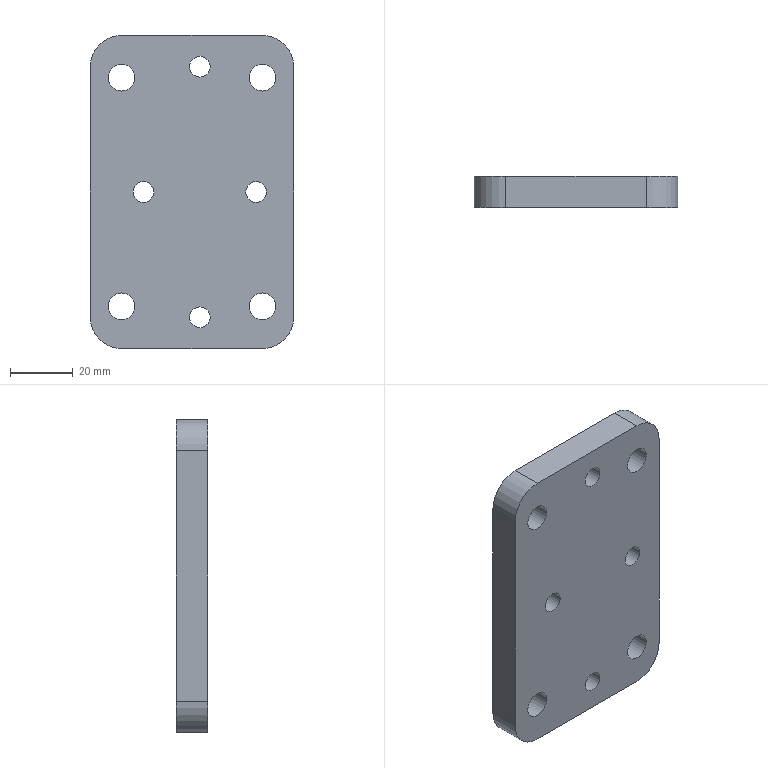Part | STEP file | JBJ-P-1006-11 | 1 solid | 22 faces | box 65 x 10 x 100 mm | volume 59980 mm3 | cylinder 12 | plane 6 | cone 4 | commonest cylinder face diameters 6.6 x4 8.5 x4 20 x4
STEP:
#1=CARTESIAN_POINT('',(0.,0.,10.));
#2=VERTEX_POINT('',#1);
#3=CARTESIAN_POINT('',(0.,0.,90.));
#4=VERTEX_POINT('',#3);
#5=CARTESIAN_POINT('',(0.,0.,0.));
#6=DIRECTION('',(0.,0.,1.));
#7=VECTOR('',#6,1000.);
#8=LINE('',#5,#7);
#9=EDGE_CURVE('',#2,#4,#8,.T.);
#10=ORIENTED_EDGE('',*,*,#9,.T.);
#11=CARTESIAN_POINT('',(0.,10.,90.));
#12=VERTEX_POINT('',#11);
#13=CARTESIAN_POINT('',(0.,10.,90.));
#14=DIRECTION('',(0.,1.,0.));
#15=VECTOR('',#14,1000.);
#16=LINE('',#13,#15);
#17=EDGE_CURVE('',#4,#12,#16,.T.);
#18=ORIENTED_EDGE('',*,*,#17,.T.);
#19=CARTESIAN_POINT('',(0.,10.,10.));
#20=VERTEX_POINT('',#19);
#21=CARTESIAN_POINT('',(0.,10.,0.));
#22=DIRECTION('',(0.,0.,1.));
#23=VECTOR('',#22,1000.);
#24=LINE('',#21,#23);
#25=EDGE_CURVE('',#20,#12,#24,.T.);
#26=ORIENTED_EDGE('',*,*,#25,.F.);
#27=CARTESIAN_POINT('',(0.,10.,10.));
#28=DIRECTION('',(0.,-1.,0.));
#29=VECTOR('',#28,1000.);
#30=LINE('',#27,#29);
#31=EDGE_CURVE('',#20,#2,#30,.T.);
#32=ORIENTED_EDGE('',*,*,#31,.T.);
#33=EDGE_LOOP('',(#10,#18,#26,#32));
#34=FACE_OUTER_BOUND('',#33,.T.);
#35=CARTESIAN_POINT('',(0.,10.,0.));
#36=DIRECTION('',(1.,0.,0.));
#37=DIRECTION('',(0.,0.,-1.));
#38=AXIS2_PLACEMENT_3D('',#35,#36,#37);
#39=PLANE('',#38);
#40=ADVANCED_FACE('',(#34),#39,.F.);
#41=CARTESIAN_POINT('',(10.,10.,100.));
#42=VERTEX_POINT('',#41);
#43=CARTESIAN_POINT('',(55.,10.,100.));
#44=VERTEX_POINT('',#43);
#45=CARTESIAN_POINT('',(0.,10.,100.));
#46=DIRECTION('',(1.,0.,0.));
#47=VECTOR('',#46,1000.);
#48=LINE('',#45,#47);
#49=EDGE_CURVE('',#42,#44,#48,.T.);
#50=ORIENTED_EDGE('',*,*,#49,.F.);
#51=CARTESIAN_POINT('',(10.,0.,100.));
#52=VERTEX_POINT('',#51);
#53=CARTESIAN_POINT('',(10.,10.,100.));
#54=DIRECTION('',(0.,-1.,0.));
#55=VECTOR('',#54,1000.);
#56=LINE('',#53,#55);
#57=EDGE_CURVE('',#42,#52,#56,.T.);
#58=ORIENTED_EDGE('',*,*,#57,.T.);
#59=CARTESIAN_POINT('',(55.,0.,100.));
#60=VERTEX_POINT('',#59);
#61=CARTESIAN_POINT('',(0.,0.,100.));
#62=DIRECTION('',(1.,0.,0.));
#63=VECTOR('',#62,1000.);
#64=LINE('',#61,#63);
#65=EDGE_CURVE('',#52,#60,#64,.T.);
#66=ORIENTED_EDGE('',*,*,#65,.T.);
#67=CARTESIAN_POINT('',(55.,10.,100.));
#68=DIRECTION('',(0.,1.,0.));
#69=VECTOR('',#68,1000.);
#70=LINE('',#67,#69);
#71=EDGE_CURVE('',#60,#44,#70,.T.);
#72=ORIENTED_EDGE('',*,*,#71,.T.);
#73=EDGE_LOOP('',(#50,#58,#66,#72));
#74=FACE_OUTER_BOUND('',#73,.T.);
#75=CARTESIAN_POINT('',(0.,10.,100.));
#76=DIRECTION('',(0.,0.,-1.));
#77=DIRECTION('',(-1.,0.,0.));
#78=AXIS2_PLACEMENT_3D('',#75,#76,#77);
#79=PLANE('',#78);
#80=ADVANCED_FACE('',(#74),#79,.F.);
#81=CARTESIAN_POINT('',(65.,10.,90.));
#82=VERTEX_POINT('',#81);
#83=CARTESIAN_POINT('',(65.,10.,10.));
#84=VERTEX_POINT('',#83);
#85=CARTESIAN_POINT('',(65.,10.,0.));
#86=DIRECTION('',(0.,0.,-1.));
#87=VECTOR('',#86,1000.);
#88=LINE('',#85,#87);
#89=EDGE_CURVE('',#82,#84,#88,.T.);
#90=ORIENTED_EDGE('',*,*,#89,.F.);
#91=CARTESIAN_POINT('',(65.,0.,90.));
#92=VERTEX_POINT('',#91);
#93=CARTESIAN_POINT('',(65.,10.,90.));
#94=DIRECTION('',(0.,-1.,0.));
#95=VECTOR('',#94,1000.);
#96=LINE('',#93,#95);
#97=EDGE_CURVE('',#82,#92,#96,.T.);
#98=ORIENTED_EDGE('',*,*,#97,.T.);
#99=CARTESIAN_POINT('',(65.,0.,10.));
#100=VERTEX_POINT('',#99);
#101=CARTESIAN_POINT('',(65.,0.,0.));
#102=DIRECTION('',(0.,0.,-1.));
#103=VECTOR('',#102,1000.);
#104=LINE('',#101,#103);
#105=EDGE_CURVE('',#92,#100,#104,.T.);
#106=ORIENTED_EDGE('',*,*,#105,.T.);
#107=CARTESIAN_POINT('',(65.,10.,10.));
#108=DIRECTION('',(0.,1.,0.));
#109=VECTOR('',#108,1000.);
#110=LINE('',#107,#109);
#111=EDGE_CURVE('',#100,#84,#110,.T.);
#112=ORIENTED_EDGE('',*,*,#111,.T.);
#113=EDGE_LOOP('',(#90,#98,#106,#112));
#114=FACE_OUTER_BOUND('',#113,.T.);
#115=CARTESIAN_POINT('',(65.,10.,0.));
#116=DIRECTION('',(-1.,0.,0.));
#117=DIRECTION('',(0.,0.,1.));
#118=AXIS2_PLACEMENT_3D('',#115,#116,#117);
#119=PLANE('',#118);
#120=ADVANCED_FACE('',(#114),#119,.F.);
#121=CARTESIAN_POINT('',(55.,10.,0.));
#122=VERTEX_POINT('',#121);
#123=CARTESIAN_POINT('',(10.,10.,0.));
#124=VERTEX_POINT('',#123);
#125=CARTESIAN_POINT('',(0.,10.,0.));
#126=DIRECTION('',(-1.,0.,0.));
#127=VECTOR('',#126,1000.);
#128=LINE('',#125,#127);
#129=EDGE_CURVE('',#122,#124,#128,.T.);
#130=ORIENTED_EDGE('',*,*,#129,.F.);
#131=CARTESIAN_POINT('',(55.,0.,0.));
#132=VERTEX_POINT('',#131);
#133=CARTESIAN_POINT('',(55.,10.,0.));
#134=DIRECTION('',(0.,-1.,0.));
#135=VECTOR('',#134,1000.);
#136=LINE('',#133,#135);
#137=EDGE_CURVE('',#122,#132,#136,.T.);
#138=ORIENTED_EDGE('',*,*,#137,.T.);
#139=CARTESIAN_POINT('',(10.,0.,0.));
#140=VERTEX_POINT('',#139);
#141=CARTESIAN_POINT('',(0.,0.,0.));
#142=DIRECTION('',(-1.,0.,0.));
#143=VECTOR('',#142,1000.);
#144=LINE('',#141,#143);
#145=EDGE_CURVE('',#132,#140,#144,.T.);
#146=ORIENTED_EDGE('',*,*,#145,.T.);
#147=CARTESIAN_POINT('',(10.,10.,0.));
#148=DIRECTION('',(0.,1.,0.));
#149=VECTOR('',#148,1000.);
#150=LINE('',#147,#149);
#151=EDGE_CURVE('',#140,#124,#150,.T.);
#152=ORIENTED_EDGE('',*,*,#151,.T.);
#153=EDGE_LOOP('',(#130,#138,#146,#152));
#154=FACE_OUTER_BOUND('',#153,.T.);
#155=CARTESIAN_POINT('',(0.,10.,0.));
#156=DIRECTION('',(0.,0.,1.));
#157=DIRECTION('',(1.,0.,0.));
#158=AXIS2_PLACEMENT_3D('',#155,#156,#157);
#159=PLANE('',#158);
#160=ADVANCED_FACE('',(#154),#159,.F.);
#161=CARTESIAN_POINT('',(17.,10.,56.4));
#162=VERTEX_POINT('',#161);
#163=CARTESIAN_POINT('',(17.,10.,50.));
#164=DIRECTION('',(0.,1.,0.));
#165=DIRECTION('',(0.,0.,1.));
#166=AXIS2_PLACEMENT_3D('',#163,#164,#165);
#167=CIRCLE('',#166,6.4);
#168=EDGE_CURVE('',#162,#162,#167,.T.);
#169=ORIENTED_EDGE('',*,*,#168,.F.);
#170=EDGE_LOOP('',(#169));
#171=FACE_BOUND('',#170,.T.);
#172=CARTESIAN_POINT('',(35.,10.,16.4));
#173=VERTEX_POINT('',#172);
#174=CARTESIAN_POINT('',(35.,10.,10.));
#175=DIRECTION('',(0.,1.,0.));
#176=DIRECTION('',(0.,0.,1.));
#177=AXIS2_PLACEMENT_3D('',#174,#175,#176);
#178=CIRCLE('',#177,6.4);
#179=EDGE_CURVE('',#173,#173,#178,.T.);
#180=ORIENTED_EDGE('',*,*,#179,.F.);
#181=EDGE_LOOP('',(#180));
#182=FACE_BOUND('',#181,.T.);
#183=CARTESIAN_POINT('',(35.,10.,96.4));
#184=VERTEX_POINT('',#183);
#185=CARTESIAN_POINT('',(35.,10.,90.));
#186=DIRECTION('',(0.,1.,0.));
#187=DIRECTION('',(0.,0.,1.));
#188=AXIS2_PLACEMENT_3D('',#185,#186,#187);
#189=CIRCLE('',#188,6.4);
#190=EDGE_CURVE('',#184,#184,#189,.T.);
#191=ORIENTED_EDGE('',*,*,#190,.F.);
#192=EDGE_LOOP('',(#191));
#193=FACE_BOUND('',#192,.T.);
#194=CARTESIAN_POINT('',(53.,10.,56.4));
#195=VERTEX_POINT('',#194);
#196=CARTESIAN_POINT('',(53.,10.,50.));
#197=DIRECTION('',(0.,1.,0.));
#198=DIRECTION('',(0.,0.,1.));
#199=AXIS2_PLACEMENT_3D('',#196,#197,#198);
#200=CIRCLE('',#199,6.4);
#201=EDGE_CURVE('',#195,#195,#200,.T.);
#202=ORIENTED_EDGE('',*,*,#201,.F.);
#203=EDGE_LOOP('',(#202));
#204=FACE_BOUND('',#203,.T.);
#205=CARTESIAN_POINT('',(10.,10.,17.75));
#206=VERTEX_POINT('',#205);
#207=CARTESIAN_POINT('',(10.,10.,13.5));
#208=DIRECTION('',(0.,1.,0.));
#209=DIRECTION('',(0.,0.,1.));
#210=AXIS2_PLACEMENT_3D('',#207,#208,#209);
#211=CIRCLE('',#210,4.25);
#212=EDGE_CURVE('',#206,#206,#211,.T.);
#213=ORIENTED_EDGE('',*,*,#212,.F.);
#214=EDGE_LOOP('',(#213));
#215=FACE_BOUND('',#214,.T.);
#216=CARTESIAN_POINT('',(55.,10.,17.75));
#217=VERTEX_POINT('',#216);
#218=CARTESIAN_POINT('',(55.,10.,13.5));
#219=DIRECTION('',(0.,1.,0.));
#220=DIRECTION('',(0.,0.,1.));
#221=AXIS2_PLACEMENT_3D('',#218,#219,#220);
#222=CIRCLE('',#221,4.25);
#223=EDGE_CURVE('',#217,#217,#222,.T.);
#224=ORIENTED_EDGE('',*,*,#223,.F.);
#225=EDGE_LOOP('',(#224));
#226=FACE_BOUND('',#225,.T.);
#227=CARTESIAN_POINT('',(55.,10.,90.75));
#228=VERTEX_POINT('',#227);
#229=CARTESIAN_POINT('',(55.,10.,86.5));
#230=DIRECTION('',(0.,1.,0.));
#231=DIRECTION('',(0.,0.,1.));
#232=AXIS2_PLACEMENT_3D('',#229,#230,#231);
#233=CIRCLE('',#232,4.25);
#234=EDGE_CURVE('',#228,#228,#233,.T.);
#235=ORIENTED_EDGE('',*,*,#234,.F.);
#236=EDGE_LOOP('',(#235));
#237=FACE_BOUND('',#236,.T.);
#238=CARTESIAN_POINT('',(10.,10.,90.75));
#239=VERTEX_POINT('',#238);
#240=CARTESIAN_POINT('',(10.,10.,86.5));
#241=DIRECTION('',(0.,1.,0.));
#242=DIRECTION('',(0.,0.,1.));
#243=AXIS2_PLACEMENT_3D('',#240,#241,#242);
#244=CIRCLE('',#243,4.25);
#245=EDGE_CURVE('',#239,#239,#244,.T.);
#246=ORIENTED_EDGE('',*,*,#245,.F.);
#247=EDGE_LOOP('',(#246));
#248=FACE_BOUND('',#247,.T.);
#249=ORIENTED_EDGE('',*,*,#25,.T.);
#250=CARTESIAN_POINT('',(10.,10.,90.));
#251=DIRECTION('',(0.,1.,0.));
#252=DIRECTION('',(0.,0.,1.));
#253=AXIS2_PLACEMENT_3D('',#250,#251,#252);
#254=CIRCLE('',#253,10.);
#255=EDGE_CURVE('',#12,#42,#254,.T.);
#256=ORIENTED_EDGE('',*,*,#255,.T.);
#257=ORIENTED_EDGE('',*,*,#49,.T.);
#258=CARTESIAN_POINT('',(55.,10.,90.));
#259=DIRECTION('',(0.,1.,0.));
#260=DIRECTION('',(0.,0.,1.));
#261=AXIS2_PLACEMENT_3D('',#258,#259,#260);
#262=CIRCLE('',#261,10.);
#263=EDGE_CURVE('',#44,#82,#262,.T.);
#264=ORIENTED_EDGE('',*,*,#263,.T.);
#265=ORIENTED_EDGE('',*,*,#89,.T.);
#266=CARTESIAN_POINT('',(55.,10.,10.));
#267=DIRECTION('',(0.,1.,0.));
#268=DIRECTION('',(0.,0.,1.));
#269=AXIS2_PLACEMENT_3D('',#266,#267,#268);
#270=CIRCLE('',#269,10.);
#271=EDGE_CURVE('',#84,#122,#270,.T.);
#272=ORIENTED_EDGE('',*,*,#271,.T.);
#273=ORIENTED_EDGE('',*,*,#129,.T.);
#274=CARTESIAN_POINT('',(10.,10.,10.));
#275=DIRECTION('',(0.,1.,0.));
#276=DIRECTION('',(0.,0.,1.));
#277=AXIS2_PLACEMENT_3D('',#274,#275,#276);
#278=CIRCLE('',#277,10.);
#279=EDGE_CURVE('',#124,#20,#278,.T.);
#280=ORIENTED_EDGE('',*,*,#279,.T.);
#281=EDGE_LOOP('',(#249,#256,#257,#264,#265,#272,#273,#280));
#282=FACE_OUTER_BOUND('',#281,.T.);
#283=CARTESIAN_POINT('',(0.,10.,0.));
#284=DIRECTION('',(0.,1.,0.));
#285=DIRECTION('',(0.,0.,1.));
#286=AXIS2_PLACEMENT_3D('',#283,#284,#285);
#287=PLANE('',#286);
#288=ADVANCED_FACE('',(#171,#182,#193,#204,#215,#226,#237,#248,#282),#287,.T.);
#289=CARTESIAN_POINT('',(17.,0.,53.3));
#290=VERTEX_POINT('',#289);
#291=CARTESIAN_POINT('',(17.,0.,50.));
#292=DIRECTION('',(0.,1.,0.));
#293=DIRECTION('',(0.,0.,1.));
#294=AXIS2_PLACEMENT_3D('',#291,#292,#293);
#295=CIRCLE('',#294,3.3);
#296=EDGE_CURVE('',#290,#290,#295,.T.);
#297=ORIENTED_EDGE('',*,*,#296,.T.);
#298=EDGE_LOOP('',(#297));
#299=FACE_BOUND('',#298,.T.);
#300=CARTESIAN_POINT('',(35.,0.,13.3));
#301=VERTEX_POINT('',#300);
#302=CARTESIAN_POINT('',(35.,0.,10.));
#303=DIRECTION('',(0.,1.,0.));
#304=DIRECTION('',(0.,0.,1.));
#305=AXIS2_PLACEMENT_3D('',#302,#303,#304);
#306=CIRCLE('',#305,3.3);
#307=EDGE_CURVE('',#301,#301,#306,.T.);
#308=ORIENTED_EDGE('',*,*,#307,.T.);
#309=EDGE_LOOP('',(#308));
#310=FACE_BOUND('',#309,.T.);
#311=CARTESIAN_POINT('',(35.,0.,93.3));
#312=VERTEX_POINT('',#311);
#313=CARTESIAN_POINT('',(35.,0.,90.));
#314=DIRECTION('',(0.,1.,0.));
#315=DIRECTION('',(0.,0.,1.));
#316=AXIS2_PLACEMENT_3D('',#313,#314,#315);
#317=CIRCLE('',#316,3.3);
#318=EDGE_CURVE('',#312,#312,#317,.T.);
#319=ORIENTED_EDGE('',*,*,#318,.T.);
#320=EDGE_LOOP('',(#319));
#321=FACE_BOUND('',#320,.T.);
#322=CARTESIAN_POINT('',(53.,0.,53.3));
#323=VERTEX_POINT('',#322);
#324=CARTESIAN_POINT('',(53.,0.,50.));
#325=DIRECTION('',(0.,1.,0.));
#326=DIRECTION('',(0.,0.,1.));
#327=AXIS2_PLACEMENT_3D('',#324,#325,#326);
#328=CIRCLE('',#327,3.3);
#329=EDGE_CURVE('',#323,#323,#328,.T.);
#330=ORIENTED_EDGE('',*,*,#329,.T.);
#331=EDGE_LOOP('',(#330));
#332=FACE_BOUND('',#331,.T.);
#333=CARTESIAN_POINT('',(10.,0.,17.75));
#334=VERTEX_POINT('',#333);
#335=CARTESIAN_POINT('',(10.,0.,13.5));
#336=DIRECTION('',(0.,1.,0.));
#337=DIRECTION('',(0.,0.,1.));
#338=AXIS2_PLACEMENT_3D('',#335,#336,#337);
#339=CIRCLE('',#338,4.25);
#340=EDGE_CURVE('',#334,#334,#339,.T.);
#341=ORIENTED_EDGE('',*,*,#340,.T.);
#342=EDGE_LOOP('',(#341));
#343=FACE_BOUND('',#342,.T.);
#344=CARTESIAN_POINT('',(55.,0.,17.75));
#345=VERTEX_POINT('',#344);
#346=CARTESIAN_POINT('',(55.,0.,13.5));
#347=DIRECTION('',(0.,1.,0.));
#348=DIRECTION('',(0.,0.,1.));
#349=AXIS2_PLACEMENT_3D('',#346,#347,#348);
#350=CIRCLE('',#349,4.25);
#351=EDGE_CURVE('',#345,#345,#350,.T.);
#352=ORIENTED_EDGE('',*,*,#351,.T.);
#353=EDGE_LOOP('',(#352));
#354=FACE_BOUND('',#353,.T.);
#355=CARTESIAN_POINT('',(55.,0.,90.75));
#356=VERTEX_POINT('',#355);
#357=CARTESIAN_POINT('',(55.,0.,86.5));
#358=DIRECTION('',(0.,1.,0.));
#359=DIRECTION('',(0.,0.,1.));
#360=AXIS2_PLACEMENT_3D('',#357,#358,#359);
#361=CIRCLE('',#360,4.25);
#362=EDGE_CURVE('',#356,#356,#361,.T.);
#363=ORIENTED_EDGE('',*,*,#362,.T.);
#364=EDGE_LOOP('',(#363));
#365=FACE_BOUND('',#364,.T.);
#366=CARTESIAN_POINT('',(10.,0.,90.75));
#367=VERTEX_POINT('',#366);
#368=CARTESIAN_POINT('',(10.,0.,86.5));
#369=DIRECTION('',(0.,1.,0.));
#370=DIRECTION('',(0.,0.,1.));
#371=AXIS2_PLACEMENT_3D('',#368,#369,#370);
#372=CIRCLE('',#371,4.25);
#373=EDGE_CURVE('',#367,#367,#372,.T.);
#374=ORIENTED_EDGE('',*,*,#373,.T.);
#375=EDGE_LOOP('',(#374));
#376=FACE_BOUND('',#375,.T.);
#377=ORIENTED_EDGE('',*,*,#65,.F.);
#378=CARTESIAN_POINT('',(10.,0.,90.));
#379=DIRECTION('',(0.,-1.,0.));
#380=DIRECTION('',(0.,0.,1.));
#381=AXIS2_PLACEMENT_3D('',#378,#379,#380);
#382=CIRCLE('',#381,10.);
#383=EDGE_CURVE('',#52,#4,#382,.T.);
#384=ORIENTED_EDGE('',*,*,#383,.T.);
#385=ORIENTED_EDGE('',*,*,#9,.F.);
#386=CARTESIAN_POINT('',(10.,0.,10.));
#387=DIRECTION('',(0.,-1.,0.));
#388=DIRECTION('',(0.,0.,1.));
#389=AXIS2_PLACEMENT_3D('',#386,#387,#388);
#390=CIRCLE('',#389,10.);
#391=EDGE_CURVE('',#2,#140,#390,.T.);
#392=ORIENTED_EDGE('',*,*,#391,.T.);
#393=ORIENTED_EDGE('',*,*,#145,.F.);
#394=CARTESIAN_POINT('',(55.,0.,10.));
#395=DIRECTION('',(0.,-1.,0.));
#396=DIRECTION('',(0.,0.,1.));
#397=AXIS2_PLACEMENT_3D('',#394,#395,#396);
#398=CIRCLE('',#397,10.);
#399=EDGE_CURVE('',#132,#100,#398,.T.);
#400=ORIENTED_EDGE('',*,*,#399,.T.);
#401=ORIENTED_EDGE('',*,*,#105,.F.);
#402=CARTESIAN_POINT('',(55.,0.,90.));
#403=DIRECTION('',(0.,-1.,0.));
#404=DIRECTION('',(0.,0.,1.));
#405=AXIS2_PLACEMENT_3D('',#402,#403,#404);
#406=CIRCLE('',#405,10.);
#407=EDGE_CURVE('',#92,#60,#406,.T.);
#408=ORIENTED_EDGE('',*,*,#407,.T.);
#409=EDGE_LOOP('',(#377,#384,#385,#392,#393,#400,#401,#408));
#410=FACE_OUTER_BOUND('',#409,.T.);
#411=CARTESIAN_POINT('',(0.,0.,0.));
#412=DIRECTION('',(0.,1.,0.));
#413=DIRECTION('',(0.,0.,1.));
#414=AXIS2_PLACEMENT_3D('',#411,#412,#413);
#415=PLANE('',#414);
#416=ADVANCED_FACE('',(#299,#310,#321,#332,#343,#354,#365,#376,#410),#415,.F.);
#417=ORIENTED_EDGE('',*,*,#255,.F.);
#418=ORIENTED_EDGE('',*,*,#17,.F.);
#419=ORIENTED_EDGE('',*,*,#383,.F.);
#420=ORIENTED_EDGE('',*,*,#57,.F.);
#421=EDGE_LOOP('',(#417,#418,#419,#420));
#422=FACE_OUTER_BOUND('',#421,.T.);
#423=CARTESIAN_POINT('',(10.,10.,90.));
#424=DIRECTION('',(0.,-1.,0.));
#425=DIRECTION('',(0.,0.,-1.));
#426=AXIS2_PLACEMENT_3D('',#423,#424,#425);
#427=CYLINDRICAL_SURFACE('',#426,10.);
#428=ADVANCED_FACE('',(#422),#427,.T.);
#429=ORIENTED_EDGE('',*,*,#263,.F.);
#430=ORIENTED_EDGE('',*,*,#71,.F.);
#431=ORIENTED_EDGE('',*,*,#407,.F.);
#432=ORIENTED_EDGE('',*,*,#97,.F.);
#433=EDGE_LOOP('',(#429,#430,#431,#432));
#434=FACE_OUTER_BOUND('',#433,.T.);
#435=CARTESIAN_POINT('',(55.,10.,90.));
#436=DIRECTION('',(0.,-1.,0.));
#437=DIRECTION('',(0.,0.,-1.));
#438=AXIS2_PLACEMENT_3D('',#435,#436,#437);
#439=CYLINDRICAL_SURFACE('',#438,10.);
#440=ADVANCED_FACE('',(#434),#439,.T.);
#441=ORIENTED_EDGE('',*,*,#271,.F.);
#442=ORIENTED_EDGE('',*,*,#111,.F.);
#443=ORIENTED_EDGE('',*,*,#399,.F.);
#444=ORIENTED_EDGE('',*,*,#137,.F.);
#445=EDGE_LOOP('',(#441,#442,#443,#444));
#446=FACE_OUTER_BOUND('',#445,.T.);
#447=CARTESIAN_POINT('',(55.,10.,10.));
#448=DIRECTION('',(0.,-1.,0.));
#449=DIRECTION('',(0.,0.,-1.));
#450=AXIS2_PLACEMENT_3D('',#447,#448,#449);
#451=CYLINDRICAL_SURFACE('',#450,10.);
#452=ADVANCED_FACE('',(#446),#451,.T.);
#453=ORIENTED_EDGE('',*,*,#279,.F.);
#454=ORIENTED_EDGE('',*,*,#151,.F.);
#455=ORIENTED_EDGE('',*,*,#391,.F.);
#456=ORIENTED_EDGE('',*,*,#31,.F.);
#457=EDGE_LOOP('',(#453,#454,#455,#456));
#458=FACE_OUTER_BOUND('',#457,.T.);
#459=CARTESIAN_POINT('',(10.,10.,10.));
#460=DIRECTION('',(0.,-1.,0.));
#461=DIRECTION('',(0.,0.,-1.));
#462=AXIS2_PLACEMENT_3D('',#459,#460,#461);
#463=CYLINDRICAL_SURFACE('',#462,10.);
#464=ADVANCED_FACE('',(#458),#463,.T.);
#465=ORIENTED_EDGE('',*,*,#245,.T.);
#466=EDGE_LOOP('',(#465));
#467=FACE_OUTER_BOUND('',#466,.T.);
#468=ORIENTED_EDGE('',*,*,#373,.F.);
#469=EDGE_LOOP('',(#468));
#470=FACE_OUTER_BOUND('',#469,.T.);
#471=CARTESIAN_POINT('',(10.,10.,86.5));
#472=DIRECTION('',(0.,1.,0.));
#473=DIRECTION('',(0.,0.,1.));
#474=AXIS2_PLACEMENT_3D('',#471,#472,#473);
#475=CYLINDRICAL_SURFACE('',#474,4.25);
#476=ADVANCED_FACE('',(#467,#470),#475,.F.);
#477=ORIENTED_EDGE('',*,*,#234,.T.);
#478=EDGE_LOOP('',(#477));
#479=FACE_OUTER_BOUND('',#478,.T.);
#480=ORIENTED_EDGE('',*,*,#362,.F.);
#481=EDGE_LOOP('',(#480));
#482=FACE_OUTER_BOUND('',#481,.T.);
#483=CARTESIAN_POINT('',(55.,10.,86.5));
#484=DIRECTION('',(0.,1.,0.));
#485=DIRECTION('',(0.,0.,1.));
#486=AXIS2_PLACEMENT_3D('',#483,#484,#485);
#487=CYLINDRICAL_SURFACE('',#486,4.25);
#488=ADVANCED_FACE('',(#479,#482),#487,.F.);
#489=ORIENTED_EDGE('',*,*,#223,.T.);
#490=EDGE_LOOP('',(#489));
#491=FACE_OUTER_BOUND('',#490,.T.);
#492=ORIENTED_EDGE('',*,*,#351,.F.);
#493=EDGE_LOOP('',(#492));
#494=FACE_OUTER_BOUND('',#493,.T.);
#495=CARTESIAN_POINT('',(55.,10.,13.5));
#496=DIRECTION('',(0.,1.,0.));
#497=DIRECTION('',(0.,0.,1.));
#498=AXIS2_PLACEMENT_3D('',#495,#496,#497);
#499=CYLINDRICAL_SURFACE('',#498,4.25);
#500=ADVANCED_FACE('',(#491,#494),#499,.F.);
#501=ORIENTED_EDGE('',*,*,#212,.T.);
#502=EDGE_LOOP('',(#501));
#503=FACE_OUTER_BOUND('',#502,.T.);
#504=ORIENTED_EDGE('',*,*,#340,.F.);
#505=EDGE_LOOP('',(#504));
#506=FACE_OUTER_BOUND('',#505,.T.);
#507=CARTESIAN_POINT('',(10.,10.,13.5));
#508=DIRECTION('',(0.,1.,0.));
#509=DIRECTION('',(0.,0.,1.));
#510=AXIS2_PLACEMENT_3D('',#507,#508,#509);
#511=CYLINDRICAL_SURFACE('',#510,4.25);
#512=ADVANCED_FACE('',(#503,#506),#511,.F.);
#513=CARTESIAN_POINT('',(53.,6.9,53.3));
#514=VERTEX_POINT('',#513);
#515=CARTESIAN_POINT('',(53.,6.9,50.));
#516=DIRECTION('',(0.,1.,0.));
#517=DIRECTION('',(0.,0.,1.));
#518=AXIS2_PLACEMENT_3D('',#515,#516,#517);
#519=CIRCLE('',#518,3.3);
#520=EDGE_CURVE('',#514,#514,#519,.T.);
#521=ORIENTED_EDGE('',*,*,#520,.T.);
#522=EDGE_LOOP('',(#521));
#523=FACE_OUTER_BOUND('',#522,.T.);
#524=ORIENTED_EDGE('',*,*,#329,.F.);
#525=EDGE_LOOP('',(#524));
#526=FACE_OUTER_BOUND('',#525,.T.);
#527=CARTESIAN_POINT('',(53.,10.,50.));
#528=DIRECTION('',(0.,1.,0.));
#529=DIRECTION('',(0.,0.,1.));
#530=AXIS2_PLACEMENT_3D('',#527,#528,#529);
#531=CYLINDRICAL_SURFACE('',#530,3.3);
#532=ADVANCED_FACE('',(#523,#526),#531,.F.);
#533=ORIENTED_EDGE('',*,*,#520,.F.);
#534=EDGE_LOOP('',(#533));
#535=FACE_BOUND('',#534,.T.);
#536=ORIENTED_EDGE('',*,*,#201,.T.);
#537=EDGE_LOOP('',(#536));
#538=FACE_OUTER_BOUND('',#537,.T.);
#539=CARTESIAN_POINT('',(53.,10.,50.));
#540=DIRECTION('',(0.,1.,0.));
#541=DIRECTION('',(0.,0.,1.));
#542=AXIS2_PLACEMENT_3D('',#539,#540,#541);
#543=CONICAL_SURFACE('',#542,6.4,0.7854);
#544=ADVANCED_FACE('',(#535,#538),#543,.F.);
#545=CARTESIAN_POINT('',(35.,6.9,93.3));
#546=VERTEX_POINT('',#545);
#547=CARTESIAN_POINT('',(35.,6.9,90.));
#548=DIRECTION('',(0.,1.,0.));
#549=DIRECTION('',(0.,0.,1.));
#550=AXIS2_PLACEMENT_3D('',#547,#548,#549);
#551=CIRCLE('',#550,3.3);
#552=EDGE_CURVE('',#546,#546,#551,.T.);
#553=ORIENTED_EDGE('',*,*,#552,.T.);
#554=EDGE_LOOP('',(#553));
#555=FACE_OUTER_BOUND('',#554,.T.);
#556=ORIENTED_EDGE('',*,*,#318,.F.);
#557=EDGE_LOOP('',(#556));
#558=FACE_OUTER_BOUND('',#557,.T.);
#559=CARTESIAN_POINT('',(35.,10.,90.));
#560=DIRECTION('',(0.,1.,0.));
#561=DIRECTION('',(0.,0.,1.));
#562=AXIS2_PLACEMENT_3D('',#559,#560,#561);
#563=CYLINDRICAL_SURFACE('',#562,3.3);
#564=ADVANCED_FACE('',(#555,#558),#563,.F.);
#565=ORIENTED_EDGE('',*,*,#552,.F.);
#566=EDGE_LOOP('',(#565));
#567=FACE_BOUND('',#566,.T.);
#568=ORIENTED_EDGE('',*,*,#190,.T.);
#569=EDGE_LOOP('',(#568));
#570=FACE_OUTER_BOUND('',#569,.T.);
#571=CARTESIAN_POINT('',(35.,10.,90.));
#572=DIRECTION('',(0.,1.,0.));
#573=DIRECTION('',(0.,0.,1.));
#574=AXIS2_PLACEMENT_3D('',#571,#572,#573);
#575=CONICAL_SURFACE('',#574,6.4,0.7854);
#576=ADVANCED_FACE('',(#567,#570),#575,.F.);
#577=CARTESIAN_POINT('',(35.,6.9,13.3));
#578=VERTEX_POINT('',#577);
#579=CARTESIAN_POINT('',(35.,6.9,10.));
#580=DIRECTION('',(0.,1.,0.));
#581=DIRECTION('',(0.,0.,1.));
#582=AXIS2_PLACEMENT_3D('',#579,#580,#581);
#583=CIRCLE('',#582,3.3);
#584=EDGE_CURVE('',#578,#578,#583,.T.);
#585=ORIENTED_EDGE('',*,*,#584,.T.);
#586=EDGE_LOOP('',(#585));
#587=FACE_OUTER_BOUND('',#586,.T.);
#588=ORIENTED_EDGE('',*,*,#307,.F.);
#589=EDGE_LOOP('',(#588));
#590=FACE_OUTER_BOUND('',#589,.T.);
#591=CARTESIAN_POINT('',(35.,10.,10.));
#592=DIRECTION('',(0.,1.,0.));
#593=DIRECTION('',(0.,0.,1.));
#594=AXIS2_PLACEMENT_3D('',#591,#592,#593);
#595=CYLINDRICAL_SURFACE('',#594,3.3);
#596=ADVANCED_FACE('',(#587,#590),#595,.F.);
#597=ORIENTED_EDGE('',*,*,#584,.F.);
#598=EDGE_LOOP('',(#597));
#599=FACE_BOUND('',#598,.T.);
#600=ORIENTED_EDGE('',*,*,#179,.T.);
#601=EDGE_LOOP('',(#600));
#602=FACE_OUTER_BOUND('',#601,.T.);
#603=CARTESIAN_POINT('',(35.,10.,10.));
#604=DIRECTION('',(0.,1.,0.));
#605=DIRECTION('',(0.,0.,1.));
#606=AXIS2_PLACEMENT_3D('',#603,#604,#605);
#607=CONICAL_SURFACE('',#606,6.4,0.7854);
#608=ADVANCED_FACE('',(#599,#602),#607,.F.);
#609=CARTESIAN_POINT('',(17.,6.9,53.3));
#610=VERTEX_POINT('',#609);
#611=CARTESIAN_POINT('',(17.,6.9,50.));
#612=DIRECTION('',(0.,1.,0.));
#613=DIRECTION('',(0.,0.,1.));
#614=AXIS2_PLACEMENT_3D('',#611,#612,#613);
#615=CIRCLE('',#614,3.3);
#616=EDGE_CURVE('',#610,#610,#615,.T.);
#617=ORIENTED_EDGE('',*,*,#616,.T.);
#618=EDGE_LOOP('',(#617));
#619=FACE_OUTER_BOUND('',#618,.T.);
#620=ORIENTED_EDGE('',*,*,#296,.F.);
#621=EDGE_LOOP('',(#620));
#622=FACE_OUTER_BOUND('',#621,.T.);
#623=CARTESIAN_POINT('',(17.,10.,50.));
#624=DIRECTION('',(0.,1.,0.));
#625=DIRECTION('',(0.,0.,1.));
#626=AXIS2_PLACEMENT_3D('',#623,#624,#625);
#627=CYLINDRICAL_SURFACE('',#626,3.3);
#628=ADVANCED_FACE('',(#619,#622),#627,.F.);
#629=ORIENTED_EDGE('',*,*,#616,.F.);
#630=EDGE_LOOP('',(#629));
#631=FACE_BOUND('',#630,.T.);
#632=ORIENTED_EDGE('',*,*,#168,.T.);
#633=EDGE_LOOP('',(#632));
#634=FACE_OUTER_BOUND('',#633,.T.);
#635=CARTESIAN_POINT('',(17.,10.,50.));
#636=DIRECTION('',(0.,1.,0.));
#637=DIRECTION('',(0.,0.,1.));
#638=AXIS2_PLACEMENT_3D('',#635,#636,#637);
#639=CONICAL_SURFACE('',#638,6.4,0.7854);
#640=ADVANCED_FACE('',(#631,#634),#639,.F.);
#641=CLOSED_SHELL('',(#40,#80,#120,#160,#288,#416,#428,#440,#452,#464,#476,#488,#500,#512,#532,#544,#564,#576,#596,#608,#628,#640));
#642=MANIFOLD_SOLID_BREP('',#641);
#643=CARTESIAN_POINT('',(0.,0.,0.));
#644=DIRECTION('',(0.,0.,1.));
#645=DIRECTION('',(1.,0.,0.));
#646=AXIS2_PLACEMENT_3D('',#643,#644,#645);
#647=(LENGTH_UNIT()NAMED_UNIT(*)SI_UNIT(.MILLI.,.METRE.));
#648=UNCERTAINTY_MEASURE_WITH_UNIT(LENGTH_MEASURE(0.00001),#647,'','');
#649=(NAMED_UNIT(*)PLANE_ANGLE_UNIT()SI_UNIT($,.RADIAN.));
#650=(NAMED_UNIT(*)SI_UNIT($,.STERADIAN.)SOLID_ANGLE_UNIT());
#651=(GEOMETRIC_REPRESENTATION_CONTEXT(3)GLOBAL_UNCERTAINTY_ASSIGNED_CONTEXT((#648))GLOBAL_UNIT_ASSIGNED_CONTEXT((#647,#649,#650))REPRESENTATION_CONTEXT('',''));
#652=ADVANCED_BREP_SHAPE_REPRESENTATION('',(#642,#646),#651);